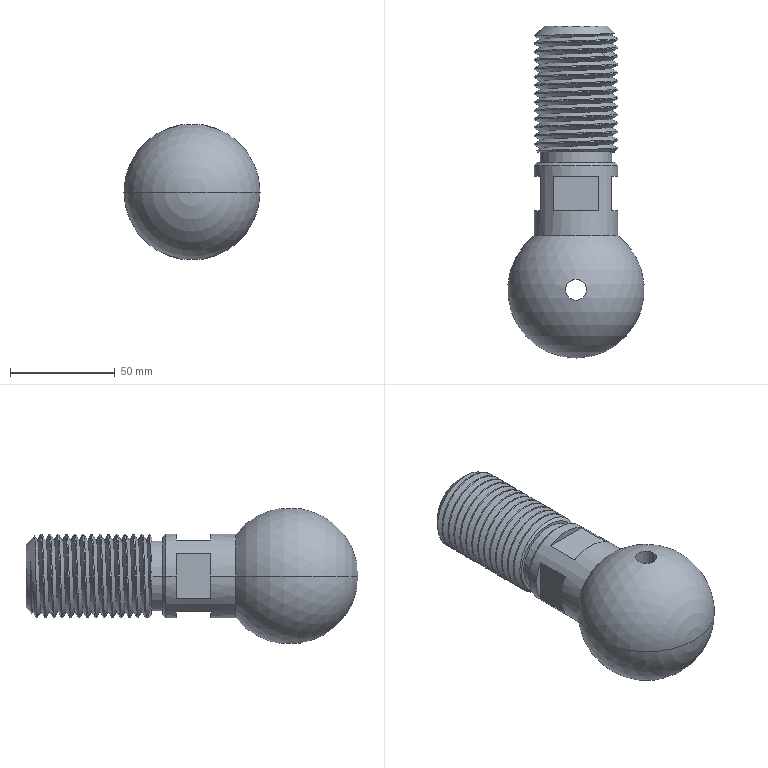Part | Creo | features CUT 7, CURVE 3, DATUM PLANE 3, CHAMFER 2, COORDINATE SYSTEM 1, PATTERN 1, PROTRUSION 1 | 1 solid | 63 faces | box 65 x 158.117 x 64.226 mm | volume 245084 mm3 | cylinder 32 | plane 16 | spline 8 | cone 5 | sphere 2 | commonest cylinder face diameters 40 x28 10 x2 34 x2